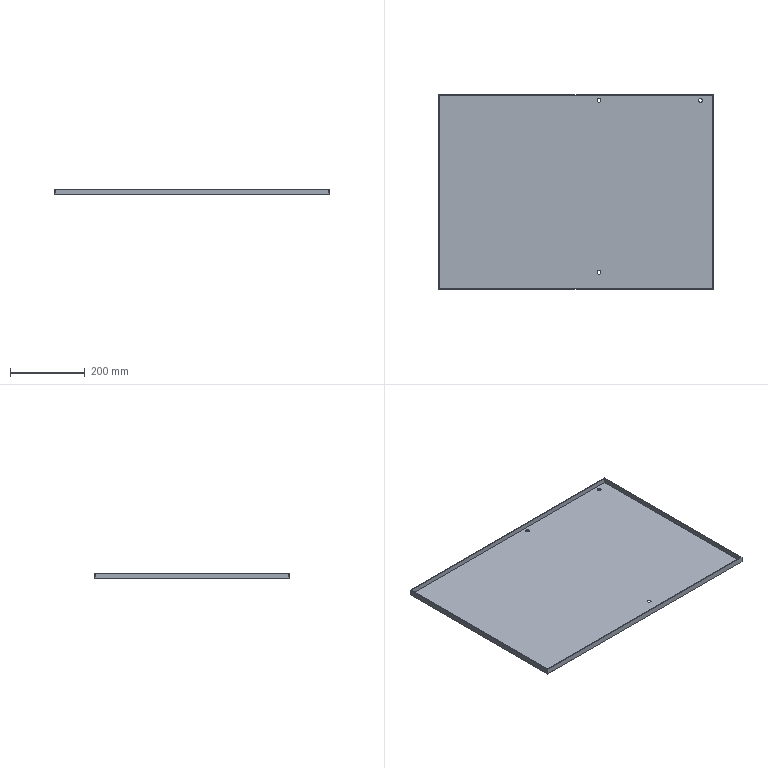Part | STEP file | 11-FGJJ-01311 | 1 solid | 17 faces | box 735 x 520 x 15 mm | volume 828981 mm3 | plane 11 | cylinder 6 | commonest cylinder face diameters 10 x6
STEP:
#1=CARTESIAN_POINT('',(56.5,245.,2.));
#2=VERTEX_POINT('',#1);
#3=CARTESIAN_POINT('',(66.5,245.,2.));
#4=VERTEX_POINT('',#3);
#5=CARTESIAN_POINT('',(61.5,245.,2.));
#6=DIRECTION('',(0.,0.,1.));
#7=DIRECTION('',(1.,0.,0.));
#8=AXIS2_PLACEMENT_3D('',#5,#6,#7);
#9=CIRCLE('',#8,5.);
#10=EDGE_CURVE('',#2,#4,#9,.T.);
#11=ORIENTED_EDGE('',*,*,#10,.T.);
#12=CARTESIAN_POINT('',(66.5,245.,0.));
#13=VERTEX_POINT('',#12);
#14=CARTESIAN_POINT('',(66.5,245.,28.));
#15=DIRECTION('',(0.,0.,-1.));
#16=VECTOR('',#15,1000.);
#17=LINE('',#14,#16);
#18=EDGE_CURVE('',#4,#13,#17,.T.);
#19=ORIENTED_EDGE('',*,*,#18,.T.);
#20=CARTESIAN_POINT('',(56.5,245.,0.));
#21=VERTEX_POINT('',#20);
#22=CARTESIAN_POINT('',(61.5,245.,0.));
#23=DIRECTION('',(0.,0.,-1.));
#24=DIRECTION('',(-1.,0.,0.));
#25=AXIS2_PLACEMENT_3D('',#22,#23,#24);
#26=CIRCLE('',#25,5.);
#27=EDGE_CURVE('',#13,#21,#26,.T.);
#28=ORIENTED_EDGE('',*,*,#27,.T.);
#29=CARTESIAN_POINT('',(56.5,245.,28.));
#30=DIRECTION('',(0.,0.,-1.));
#31=VECTOR('',#30,1000.);
#32=LINE('',#29,#31);
#33=EDGE_CURVE('',#2,#21,#32,.T.);
#34=ORIENTED_EDGE('',*,*,#33,.F.);
#35=EDGE_LOOP('',(#11,#19,#28,#34));
#36=FACE_OUTER_BOUND('',#35,.T.);
#37=CARTESIAN_POINT('',(61.5,245.,28.));
#38=DIRECTION('',(0.,0.,-1.));
#39=DIRECTION('',(-1.,0.,0.));
#40=AXIS2_PLACEMENT_3D('',#37,#38,#39);
#41=CYLINDRICAL_SURFACE('',#40,5.);
#42=ADVANCED_FACE('',(#36),#41,.F.);
#43=CARTESIAN_POINT('',(56.5,-215.,2.));
#44=VERTEX_POINT('',#43);
#45=CARTESIAN_POINT('',(66.5,-215.,2.));
#46=VERTEX_POINT('',#45);
#47=CARTESIAN_POINT('',(61.5,-215.,2.));
#48=DIRECTION('',(0.,0.,1.));
#49=DIRECTION('',(1.,0.,0.));
#50=AXIS2_PLACEMENT_3D('',#47,#48,#49);
#51=CIRCLE('',#50,5.);
#52=EDGE_CURVE('',#44,#46,#51,.T.);
#53=ORIENTED_EDGE('',*,*,#52,.T.);
#54=CARTESIAN_POINT('',(66.5,-215.,0.));
#55=VERTEX_POINT('',#54);
#56=CARTESIAN_POINT('',(66.5,-215.,28.));
#57=DIRECTION('',(0.,0.,-1.));
#58=VECTOR('',#57,1000.);
#59=LINE('',#56,#58);
#60=EDGE_CURVE('',#46,#55,#59,.T.);
#61=ORIENTED_EDGE('',*,*,#60,.T.);
#62=CARTESIAN_POINT('',(56.5,-215.,0.));
#63=VERTEX_POINT('',#62);
#64=CARTESIAN_POINT('',(61.5,-215.,0.));
#65=DIRECTION('',(0.,0.,-1.));
#66=DIRECTION('',(-1.,0.,0.));
#67=AXIS2_PLACEMENT_3D('',#64,#65,#66);
#68=CIRCLE('',#67,5.);
#69=EDGE_CURVE('',#55,#63,#68,.T.);
#70=ORIENTED_EDGE('',*,*,#69,.T.);
#71=CARTESIAN_POINT('',(56.5,-215.,28.));
#72=DIRECTION('',(0.,0.,-1.));
#73=VECTOR('',#72,1000.);
#74=LINE('',#71,#73);
#75=EDGE_CURVE('',#44,#63,#74,.T.);
#76=ORIENTED_EDGE('',*,*,#75,.F.);
#77=EDGE_LOOP('',(#53,#61,#70,#76));
#78=FACE_OUTER_BOUND('',#77,.T.);
#79=CARTESIAN_POINT('',(61.5,-215.,28.));
#80=DIRECTION('',(0.,0.,-1.));
#81=DIRECTION('',(-1.,0.,0.));
#82=AXIS2_PLACEMENT_3D('',#79,#80,#81);
#83=CYLINDRICAL_SURFACE('',#82,5.);
#84=ADVANCED_FACE('',(#78),#83,.F.);
#85=CARTESIAN_POINT('',(327.5,245.,2.));
#86=VERTEX_POINT('',#85);
#87=CARTESIAN_POINT('',(337.5,245.,2.));
#88=VERTEX_POINT('',#87);
#89=CARTESIAN_POINT('',(332.5,245.,2.));
#90=DIRECTION('',(0.,0.,1.));
#91=DIRECTION('',(1.,0.,0.));
#92=AXIS2_PLACEMENT_3D('',#89,#90,#91);
#93=CIRCLE('',#92,5.);
#94=EDGE_CURVE('',#86,#88,#93,.T.);
#95=ORIENTED_EDGE('',*,*,#94,.T.);
#96=CARTESIAN_POINT('',(337.5,245.,0.));
#97=VERTEX_POINT('',#96);
#98=CARTESIAN_POINT('',(337.5,245.,28.));
#99=DIRECTION('',(0.,0.,-1.));
#100=VECTOR('',#99,1000.);
#101=LINE('',#98,#100);
#102=EDGE_CURVE('',#88,#97,#101,.T.);
#103=ORIENTED_EDGE('',*,*,#102,.T.);
#104=CARTESIAN_POINT('',(327.5,245.,0.));
#105=VERTEX_POINT('',#104);
#106=CARTESIAN_POINT('',(332.5,245.,0.));
#107=DIRECTION('',(0.,0.,-1.));
#108=DIRECTION('',(-1.,0.,0.));
#109=AXIS2_PLACEMENT_3D('',#106,#107,#108);
#110=CIRCLE('',#109,5.);
#111=EDGE_CURVE('',#97,#105,#110,.T.);
#112=ORIENTED_EDGE('',*,*,#111,.T.);
#113=CARTESIAN_POINT('',(327.5,245.,28.));
#114=DIRECTION('',(0.,0.,-1.));
#115=VECTOR('',#114,1000.);
#116=LINE('',#113,#115);
#117=EDGE_CURVE('',#86,#105,#116,.T.);
#118=ORIENTED_EDGE('',*,*,#117,.F.);
#119=EDGE_LOOP('',(#95,#103,#112,#118));
#120=FACE_OUTER_BOUND('',#119,.T.);
#121=CARTESIAN_POINT('',(332.5,245.,28.));
#122=DIRECTION('',(0.,0.,-1.));
#123=DIRECTION('',(-1.,0.,0.));
#124=AXIS2_PLACEMENT_3D('',#121,#122,#123);
#125=CYLINDRICAL_SURFACE('',#124,5.);
#126=ADVANCED_FACE('',(#120),#125,.F.);
#127=CARTESIAN_POINT('',(367.5,-260.,0.));
#128=VERTEX_POINT('',#127);
#129=CARTESIAN_POINT('',(367.5,260.,0.));
#130=VERTEX_POINT('',#129);
#131=CARTESIAN_POINT('',(367.5,260.,0.));
#132=DIRECTION('',(0.,1.,0.));
#133=VECTOR('',#132,1000.);
#134=LINE('',#131,#133);
#135=EDGE_CURVE('',#128,#130,#134,.T.);
#136=ORIENTED_EDGE('',*,*,#135,.T.);
#137=CARTESIAN_POINT('',(367.5,260.,15.));
#138=VERTEX_POINT('',#137);
#139=CARTESIAN_POINT('',(367.5,260.,15.));
#140=DIRECTION('',(0.,0.,-1.));
#141=VECTOR('',#140,1000.);
#142=LINE('',#139,#141);
#143=EDGE_CURVE('',#138,#130,#142,.T.);
#144=ORIENTED_EDGE('',*,*,#143,.F.);
#145=CARTESIAN_POINT('',(367.5,-260.,15.));
#146=VERTEX_POINT('',#145);
#147=CARTESIAN_POINT('',(367.5,260.,15.));
#148=DIRECTION('',(0.,1.,0.));
#149=VECTOR('',#148,1000.);
#150=LINE('',#147,#149);
#151=EDGE_CURVE('',#146,#138,#150,.T.);
#152=ORIENTED_EDGE('',*,*,#151,.F.);
#153=CARTESIAN_POINT('',(367.5,-260.,15.));
#154=DIRECTION('',(0.,0.,-1.));
#155=VECTOR('',#154,1000.);
#156=LINE('',#153,#155);
#157=EDGE_CURVE('',#146,#128,#156,.T.);
#158=ORIENTED_EDGE('',*,*,#157,.T.);
#159=EDGE_LOOP('',(#136,#144,#152,#158));
#160=FACE_OUTER_BOUND('',#159,.T.);
#161=CARTESIAN_POINT('',(367.5,260.,15.));
#162=DIRECTION('',(-1.,0.,0.));
#163=DIRECTION('',(0.,-1.,0.));
#164=AXIS2_PLACEMENT_3D('',#161,#162,#163);
#165=PLANE('',#164);
#166=ADVANCED_FACE('',(#160),#165,.F.);
#167=CARTESIAN_POINT('',(-367.5,260.,0.));
#168=VERTEX_POINT('',#167);
#169=CARTESIAN_POINT('',(-367.5,260.,0.));
#170=DIRECTION('',(-1.,0.,0.));
#171=VECTOR('',#170,1000.);
#172=LINE('',#169,#171);
#173=EDGE_CURVE('',#130,#168,#172,.T.);
#174=ORIENTED_EDGE('',*,*,#173,.T.);
#175=CARTESIAN_POINT('',(-367.5,260.,15.));
#176=VERTEX_POINT('',#175);
#177=CARTESIAN_POINT('',(-367.5,260.,15.));
#178=DIRECTION('',(0.,0.,-1.));
#179=VECTOR('',#178,1000.);
#180=LINE('',#177,#179);
#181=EDGE_CURVE('',#176,#168,#180,.T.);
#182=ORIENTED_EDGE('',*,*,#181,.F.);
#183=CARTESIAN_POINT('',(-367.5,260.,15.));
#184=DIRECTION('',(-1.,0.,0.));
#185=VECTOR('',#184,1000.);
#186=LINE('',#183,#185);
#187=EDGE_CURVE('',#138,#176,#186,.T.);
#188=ORIENTED_EDGE('',*,*,#187,.F.);
#189=ORIENTED_EDGE('',*,*,#143,.T.);
#190=EDGE_LOOP('',(#174,#182,#188,#189));
#191=FACE_OUTER_BOUND('',#190,.T.);
#192=CARTESIAN_POINT('',(-367.5,260.,15.));
#193=DIRECTION('',(0.,-1.,0.));
#194=DIRECTION('',(0.,0.,-1.));
#195=AXIS2_PLACEMENT_3D('',#192,#193,#194);
#196=PLANE('',#195);
#197=ADVANCED_FACE('',(#191),#196,.F.);
#198=CARTESIAN_POINT('',(-367.5,-260.,0.));
#199=VERTEX_POINT('',#198);
#200=CARTESIAN_POINT('',(-367.5,260.,0.));
#201=DIRECTION('',(0.,-1.,0.));
#202=VECTOR('',#201,1000.);
#203=LINE('',#200,#202);
#204=EDGE_CURVE('',#168,#199,#203,.T.);
#205=ORIENTED_EDGE('',*,*,#204,.T.);
#206=CARTESIAN_POINT('',(-367.5,-260.,15.));
#207=VERTEX_POINT('',#206);
#208=CARTESIAN_POINT('',(-367.5,-260.,15.));
#209=DIRECTION('',(0.,0.,-1.));
#210=VECTOR('',#209,1000.);
#211=LINE('',#208,#210);
#212=EDGE_CURVE('',#207,#199,#211,.T.);
#213=ORIENTED_EDGE('',*,*,#212,.F.);
#214=CARTESIAN_POINT('',(-367.5,260.,15.));
#215=DIRECTION('',(0.,-1.,0.));
#216=VECTOR('',#215,1000.);
#217=LINE('',#214,#216);
#218=EDGE_CURVE('',#176,#207,#217,.T.);
#219=ORIENTED_EDGE('',*,*,#218,.F.);
#220=ORIENTED_EDGE('',*,*,#181,.T.);
#221=EDGE_LOOP('',(#205,#213,#219,#220));
#222=FACE_OUTER_BOUND('',#221,.T.);
#223=CARTESIAN_POINT('',(-367.5,260.,15.));
#224=DIRECTION('',(1.,0.,0.));
#225=DIRECTION('',(0.,1.,0.));
#226=AXIS2_PLACEMENT_3D('',#223,#224,#225);
#227=PLANE('',#226);
#228=ADVANCED_FACE('',(#222),#227,.F.);
#229=CARTESIAN_POINT('',(-367.5,-260.,0.));
#230=DIRECTION('',(1.,0.,0.));
#231=VECTOR('',#230,1000.);
#232=LINE('',#229,#231);
#233=EDGE_CURVE('',#199,#128,#232,.T.);
#234=ORIENTED_EDGE('',*,*,#233,.T.);
#235=ORIENTED_EDGE('',*,*,#157,.F.);
#236=CARTESIAN_POINT('',(-367.5,-260.,15.));
#237=DIRECTION('',(1.,0.,0.));
#238=VECTOR('',#237,1000.);
#239=LINE('',#236,#238);
#240=EDGE_CURVE('',#207,#146,#239,.T.);
#241=ORIENTED_EDGE('',*,*,#240,.F.);
#242=ORIENTED_EDGE('',*,*,#212,.T.);
#243=EDGE_LOOP('',(#234,#235,#241,#242));
#244=FACE_OUTER_BOUND('',#243,.T.);
#245=CARTESIAN_POINT('',(-367.5,-260.,15.));
#246=DIRECTION('',(0.,1.,0.));
#247=DIRECTION('',(0.,0.,1.));
#248=AXIS2_PLACEMENT_3D('',#245,#246,#247);
#249=PLANE('',#248);
#250=ADVANCED_FACE('',(#244),#249,.F.);
#251=CARTESIAN_POINT('',(365.5,-258.,15.));
#252=VERTEX_POINT('',#251);
#253=CARTESIAN_POINT('',(365.5,258.,15.));
#254=VERTEX_POINT('',#253);
#255=CARTESIAN_POINT('',(365.5,260.,15.));
#256=DIRECTION('',(0.,1.,0.));
#257=VECTOR('',#256,1000.);
#258=LINE('',#255,#257);
#259=EDGE_CURVE('',#252,#254,#258,.T.);
#260=ORIENTED_EDGE('',*,*,#259,.F.);
#261=CARTESIAN_POINT('',(-365.5,-258.,15.));
#262=VERTEX_POINT('',#261);
#263=CARTESIAN_POINT('',(-367.5,-258.,15.));
#264=DIRECTION('',(1.,0.,0.));
#265=VECTOR('',#264,1000.);
#266=LINE('',#263,#265);
#267=EDGE_CURVE('',#262,#252,#266,.T.);
#268=ORIENTED_EDGE('',*,*,#267,.F.);
#269=CARTESIAN_POINT('',(-365.5,258.,15.));
#270=VERTEX_POINT('',#269);
#271=CARTESIAN_POINT('',(-365.5,260.,15.));
#272=DIRECTION('',(0.,-1.,0.));
#273=VECTOR('',#272,1000.);
#274=LINE('',#271,#273);
#275=EDGE_CURVE('',#270,#262,#274,.T.);
#276=ORIENTED_EDGE('',*,*,#275,.F.);
#277=CARTESIAN_POINT('',(-367.5,258.,15.));
#278=DIRECTION('',(-1.,0.,0.));
#279=VECTOR('',#278,1000.);
#280=LINE('',#277,#279);
#281=EDGE_CURVE('',#254,#270,#280,.T.);
#282=ORIENTED_EDGE('',*,*,#281,.F.);
#283=EDGE_LOOP('',(#260,#268,#276,#282));
#284=FACE_BOUND('',#283,.T.);
#285=ORIENTED_EDGE('',*,*,#151,.T.);
#286=ORIENTED_EDGE('',*,*,#187,.T.);
#287=ORIENTED_EDGE('',*,*,#218,.T.);
#288=ORIENTED_EDGE('',*,*,#240,.T.);
#289=EDGE_LOOP('',(#285,#286,#287,#288));
#290=FACE_OUTER_BOUND('',#289,.T.);
#291=CARTESIAN_POINT('',(0.,0.,15.));
#292=DIRECTION('',(0.,0.,1.));
#293=DIRECTION('',(1.,0.,0.));
#294=AXIS2_PLACEMENT_3D('',#291,#292,#293);
#295=PLANE('',#294);
#296=ADVANCED_FACE('',(#284,#290),#295,.T.);
#297=CARTESIAN_POINT('',(61.5,245.,0.));
#298=DIRECTION('',(0.,0.,-1.));
#299=DIRECTION('',(-1.,0.,0.));
#300=AXIS2_PLACEMENT_3D('',#297,#298,#299);
#301=CIRCLE('',#300,5.);
#302=EDGE_CURVE('',#21,#13,#301,.T.);
#303=ORIENTED_EDGE('',*,*,#302,.F.);
#304=ORIENTED_EDGE('',*,*,#27,.F.);
#305=EDGE_LOOP('',(#303,#304));
#306=FACE_BOUND('',#305,.T.);
#307=CARTESIAN_POINT('',(61.5,-215.,0.));
#308=DIRECTION('',(0.,0.,-1.));
#309=DIRECTION('',(-1.,0.,0.));
#310=AXIS2_PLACEMENT_3D('',#307,#308,#309);
#311=CIRCLE('',#310,5.);
#312=EDGE_CURVE('',#63,#55,#311,.T.);
#313=ORIENTED_EDGE('',*,*,#312,.F.);
#314=ORIENTED_EDGE('',*,*,#69,.F.);
#315=EDGE_LOOP('',(#313,#314));
#316=FACE_BOUND('',#315,.T.);
#317=CARTESIAN_POINT('',(332.5,245.,0.));
#318=DIRECTION('',(0.,0.,-1.));
#319=DIRECTION('',(-1.,0.,0.));
#320=AXIS2_PLACEMENT_3D('',#317,#318,#319);
#321=CIRCLE('',#320,5.);
#322=EDGE_CURVE('',#105,#97,#321,.T.);
#323=ORIENTED_EDGE('',*,*,#322,.F.);
#324=ORIENTED_EDGE('',*,*,#111,.F.);
#325=EDGE_LOOP('',(#323,#324));
#326=FACE_BOUND('',#325,.T.);
#327=ORIENTED_EDGE('',*,*,#135,.F.);
#328=ORIENTED_EDGE('',*,*,#233,.F.);
#329=ORIENTED_EDGE('',*,*,#204,.F.);
#330=ORIENTED_EDGE('',*,*,#173,.F.);
#331=EDGE_LOOP('',(#327,#328,#329,#330));
#332=FACE_OUTER_BOUND('',#331,.T.);
#333=CARTESIAN_POINT('',(0.,0.,0.));
#334=DIRECTION('',(0.,0.,1.));
#335=DIRECTION('',(1.,0.,0.));
#336=AXIS2_PLACEMENT_3D('',#333,#334,#335);
#337=PLANE('',#336);
#338=ADVANCED_FACE('',(#306,#316,#326,#332),#337,.F.);
#339=CARTESIAN_POINT('',(365.5,-258.,2.));
#340=VERTEX_POINT('',#339);
#341=CARTESIAN_POINT('',(365.5,258.,2.));
#342=VERTEX_POINT('',#341);
#343=CARTESIAN_POINT('',(365.5,260.,2.));
#344=DIRECTION('',(0.,1.,0.));
#345=VECTOR('',#344,1000.);
#346=LINE('',#343,#345);
#347=EDGE_CURVE('',#340,#342,#346,.T.);
#348=ORIENTED_EDGE('',*,*,#347,.F.);
#349=CARTESIAN_POINT('',(365.5,-258.,15.));
#350=DIRECTION('',(0.,0.,-1.));
#351=VECTOR('',#350,1000.);
#352=LINE('',#349,#351);
#353=EDGE_CURVE('',#252,#340,#352,.T.);
#354=ORIENTED_EDGE('',*,*,#353,.F.);
#355=ORIENTED_EDGE('',*,*,#259,.T.);
#356=CARTESIAN_POINT('',(365.5,258.,15.));
#357=DIRECTION('',(0.,0.,-1.));
#358=VECTOR('',#357,1000.);
#359=LINE('',#356,#358);
#360=EDGE_CURVE('',#254,#342,#359,.T.);
#361=ORIENTED_EDGE('',*,*,#360,.T.);
#362=EDGE_LOOP('',(#348,#354,#355,#361));
#363=FACE_OUTER_BOUND('',#362,.T.);
#364=CARTESIAN_POINT('',(365.5,260.,15.));
#365=DIRECTION('',(-1.,0.,0.));
#366=DIRECTION('',(0.,-1.,0.));
#367=AXIS2_PLACEMENT_3D('',#364,#365,#366);
#368=PLANE('',#367);
#369=ADVANCED_FACE('',(#363),#368,.T.);
#370=CARTESIAN_POINT('',(-365.5,258.,2.));
#371=VERTEX_POINT('',#370);
#372=CARTESIAN_POINT('',(-367.5,258.,2.));
#373=DIRECTION('',(-1.,0.,0.));
#374=VECTOR('',#373,1000.);
#375=LINE('',#372,#374);
#376=EDGE_CURVE('',#342,#371,#375,.T.);
#377=ORIENTED_EDGE('',*,*,#376,.F.);
#378=ORIENTED_EDGE('',*,*,#360,.F.);
#379=ORIENTED_EDGE('',*,*,#281,.T.);
#380=CARTESIAN_POINT('',(-365.5,258.,15.));
#381=DIRECTION('',(0.,0.,-1.));
#382=VECTOR('',#381,1000.);
#383=LINE('',#380,#382);
#384=EDGE_CURVE('',#270,#371,#383,.T.);
#385=ORIENTED_EDGE('',*,*,#384,.T.);
#386=EDGE_LOOP('',(#377,#378,#379,#385));
#387=FACE_OUTER_BOUND('',#386,.T.);
#388=CARTESIAN_POINT('',(-367.5,258.,15.));
#389=DIRECTION('',(0.,-1.,0.));
#390=DIRECTION('',(0.,0.,-1.));
#391=AXIS2_PLACEMENT_3D('',#388,#389,#390);
#392=PLANE('',#391);
#393=ADVANCED_FACE('',(#387),#392,.T.);
#394=CARTESIAN_POINT('',(-365.5,-258.,2.));
#395=VERTEX_POINT('',#394);
#396=CARTESIAN_POINT('',(-365.5,260.,2.));
#397=DIRECTION('',(0.,-1.,0.));
#398=VECTOR('',#397,1000.);
#399=LINE('',#396,#398);
#400=EDGE_CURVE('',#371,#395,#399,.T.);
#401=ORIENTED_EDGE('',*,*,#400,.F.);
#402=ORIENTED_EDGE('',*,*,#384,.F.);
#403=ORIENTED_EDGE('',*,*,#275,.T.);
#404=CARTESIAN_POINT('',(-365.5,-258.,15.));
#405=DIRECTION('',(0.,0.,-1.));
#406=VECTOR('',#405,1000.);
#407=LINE('',#404,#406);
#408=EDGE_CURVE('',#262,#395,#407,.T.);
#409=ORIENTED_EDGE('',*,*,#408,.T.);
#410=EDGE_LOOP('',(#401,#402,#403,#409));
#411=FACE_OUTER_BOUND('',#410,.T.);
#412=CARTESIAN_POINT('',(-365.5,260.,15.));
#413=DIRECTION('',(1.,0.,0.));
#414=DIRECTION('',(0.,1.,0.));
#415=AXIS2_PLACEMENT_3D('',#412,#413,#414);
#416=PLANE('',#415);
#417=ADVANCED_FACE('',(#411),#416,.T.);
#418=CARTESIAN_POINT('',(-367.5,-258.,2.));
#419=DIRECTION('',(1.,0.,0.));
#420=VECTOR('',#419,1000.);
#421=LINE('',#418,#420);
#422=EDGE_CURVE('',#395,#340,#421,.T.);
#423=ORIENTED_EDGE('',*,*,#422,.F.);
#424=ORIENTED_EDGE('',*,*,#408,.F.);
#425=ORIENTED_EDGE('',*,*,#267,.T.);
#426=ORIENTED_EDGE('',*,*,#353,.T.);
#427=EDGE_LOOP('',(#423,#424,#425,#426));
#428=FACE_OUTER_BOUND('',#427,.T.);
#429=CARTESIAN_POINT('',(-367.5,-258.,15.));
#430=DIRECTION('',(0.,1.,0.));
#431=DIRECTION('',(0.,0.,1.));
#432=AXIS2_PLACEMENT_3D('',#429,#430,#431);
#433=PLANE('',#432);
#434=ADVANCED_FACE('',(#428),#433,.T.);
#435=ORIENTED_EDGE('',*,*,#10,.F.);
#436=CARTESIAN_POINT('',(61.5,245.,2.));
#437=DIRECTION('',(0.,0.,1.));
#438=DIRECTION('',(1.,0.,0.));
#439=AXIS2_PLACEMENT_3D('',#436,#437,#438);
#440=CIRCLE('',#439,5.);
#441=EDGE_CURVE('',#4,#2,#440,.T.);
#442=ORIENTED_EDGE('',*,*,#441,.F.);
#443=EDGE_LOOP('',(#435,#442));
#444=FACE_BOUND('',#443,.T.);
#445=ORIENTED_EDGE('',*,*,#52,.F.);
#446=CARTESIAN_POINT('',(61.5,-215.,2.));
#447=DIRECTION('',(0.,0.,1.));
#448=DIRECTION('',(1.,0.,0.));
#449=AXIS2_PLACEMENT_3D('',#446,#447,#448);
#450=CIRCLE('',#449,5.);
#451=EDGE_CURVE('',#46,#44,#450,.T.);
#452=ORIENTED_EDGE('',*,*,#451,.F.);
#453=EDGE_LOOP('',(#445,#452));
#454=FACE_BOUND('',#453,.T.);
#455=ORIENTED_EDGE('',*,*,#94,.F.);
#456=CARTESIAN_POINT('',(332.5,245.,2.));
#457=DIRECTION('',(0.,0.,1.));
#458=DIRECTION('',(1.,0.,0.));
#459=AXIS2_PLACEMENT_3D('',#456,#457,#458);
#460=CIRCLE('',#459,5.);
#461=EDGE_CURVE('',#88,#86,#460,.T.);
#462=ORIENTED_EDGE('',*,*,#461,.F.);
#463=EDGE_LOOP('',(#455,#462));
#464=FACE_BOUND('',#463,.T.);
#465=ORIENTED_EDGE('',*,*,#347,.T.);
#466=ORIENTED_EDGE('',*,*,#376,.T.);
#467=ORIENTED_EDGE('',*,*,#400,.T.);
#468=ORIENTED_EDGE('',*,*,#422,.T.);
#469=EDGE_LOOP('',(#465,#466,#467,#468));
#470=FACE_OUTER_BOUND('',#469,.T.);
#471=CARTESIAN_POINT('',(0.,0.,2.));
#472=DIRECTION('',(0.,0.,1.));
#473=DIRECTION('',(1.,0.,0.));
#474=AXIS2_PLACEMENT_3D('',#471,#472,#473);
#475=PLANE('',#474);
#476=ADVANCED_FACE('',(#444,#454,#464,#470),#475,.T.);
#477=ORIENTED_EDGE('',*,*,#102,.F.);
#478=ORIENTED_EDGE('',*,*,#461,.T.);
#479=ORIENTED_EDGE('',*,*,#117,.T.);
#480=ORIENTED_EDGE('',*,*,#322,.T.);
#481=EDGE_LOOP('',(#477,#478,#479,#480));
#482=FACE_OUTER_BOUND('',#481,.T.);
#483=CARTESIAN_POINT('',(332.5,245.,28.));
#484=DIRECTION('',(0.,0.,-1.));
#485=DIRECTION('',(-1.,0.,0.));
#486=AXIS2_PLACEMENT_3D('',#483,#484,#485);
#487=CYLINDRICAL_SURFACE('',#486,5.);
#488=ADVANCED_FACE('',(#482),#487,.F.);
#489=ORIENTED_EDGE('',*,*,#60,.F.);
#490=ORIENTED_EDGE('',*,*,#451,.T.);
#491=ORIENTED_EDGE('',*,*,#75,.T.);
#492=ORIENTED_EDGE('',*,*,#312,.T.);
#493=EDGE_LOOP('',(#489,#490,#491,#492));
#494=FACE_OUTER_BOUND('',#493,.T.);
#495=CARTESIAN_POINT('',(61.5,-215.,28.));
#496=DIRECTION('',(0.,0.,-1.));
#497=DIRECTION('',(-1.,0.,0.));
#498=AXIS2_PLACEMENT_3D('',#495,#496,#497);
#499=CYLINDRICAL_SURFACE('',#498,5.);
#500=ADVANCED_FACE('',(#494),#499,.F.);
#501=ORIENTED_EDGE('',*,*,#18,.F.);
#502=ORIENTED_EDGE('',*,*,#441,.T.);
#503=ORIENTED_EDGE('',*,*,#33,.T.);
#504=ORIENTED_EDGE('',*,*,#302,.T.);
#505=EDGE_LOOP('',(#501,#502,#503,#504));
#506=FACE_OUTER_BOUND('',#505,.T.);
#507=CARTESIAN_POINT('',(61.5,245.,28.));
#508=DIRECTION('',(0.,0.,-1.));
#509=DIRECTION('',(-1.,0.,0.));
#510=AXIS2_PLACEMENT_3D('',#507,#508,#509);
#511=CYLINDRICAL_SURFACE('',#510,5.);
#512=ADVANCED_FACE('',(#506),#511,.F.);
#513=CLOSED_SHELL('',(#42,#84,#126,#166,#197,#228,#250,#296,#338,#369,#393,#417,#434,#476,#488,#500,#512));
#514=MANIFOLD_SOLID_BREP('',#513);
#515=CARTESIAN_POINT('',(0.,0.,0.));
#516=DIRECTION('',(0.,0.,1.));
#517=DIRECTION('',(1.,0.,0.));
#518=AXIS2_PLACEMENT_3D('',#515,#516,#517);
#519=(LENGTH_UNIT()NAMED_UNIT(*)SI_UNIT(.MILLI.,.METRE.));
#520=UNCERTAINTY_MEASURE_WITH_UNIT(LENGTH_MEASURE(0.00001),#519,'','');
#521=(NAMED_UNIT(*)PLANE_ANGLE_UNIT()SI_UNIT($,.RADIAN.));
#522=(NAMED_UNIT(*)SI_UNIT($,.STERADIAN.)SOLID_ANGLE_UNIT());
#523=(GEOMETRIC_REPRESENTATION_CONTEXT(3)GLOBAL_UNCERTAINTY_ASSIGNED_CONTEXT((#520))GLOBAL_UNIT_ASSIGNED_CONTEXT((#519,#521,#522))REPRESENTATION_CONTEXT('',''));
#524=ADVANCED_BREP_SHAPE_REPRESENTATION('',(#514,#518),#523);